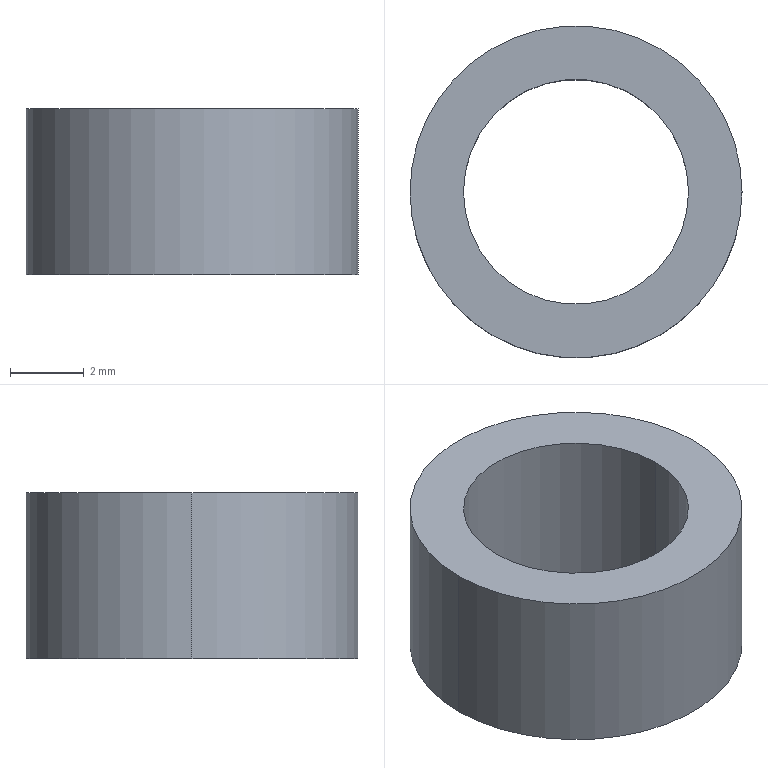Part | NX | features BREP 1 | 1 solid | 6 faces | box 9 x 9 x 4.5 mm | volume 154.767 mm3 | cylinder 4 | plane 2 | commonest cylinder face diameters 6.1 x2 9 x2
STEP:
#1=CARTESIAN_POINT('',(3.05,0.,4.5));
#2=VERTEX_POINT('',#1);
#3=CARTESIAN_POINT('',(3.05,0.,0.));
#4=VERTEX_POINT('',#3);
#5=CARTESIAN_POINT('',(3.05,0.,4.5));
#6=DIRECTION('',(0.,0.,-1.));
#7=VECTOR('',#6,1000.);
#8=LINE('',#5,#7);
#9=EDGE_CURVE('',#2,#4,#8,.T.);
#10=ORIENTED_EDGE('',*,*,#9,.F.);
#11=CARTESIAN_POINT('',(-3.05,0.,4.5));
#12=VERTEX_POINT('',#11);
#13=CARTESIAN_POINT('',(0.,0.,4.5));
#14=DIRECTION('',(0.,0.,1.));
#15=DIRECTION('',(1.,0.,0.));
#16=AXIS2_PLACEMENT_3D('',#13,#14,#15);
#17=CIRCLE('',#16,3.05);
#18=EDGE_CURVE('',#2,#12,#17,.T.);
#19=ORIENTED_EDGE('',*,*,#18,.T.);
#20=CARTESIAN_POINT('',(-3.05,0.,0.));
#21=VERTEX_POINT('',#20);
#22=CARTESIAN_POINT('',(-3.05,0.,4.5));
#23=DIRECTION('',(0.,0.,-1.));
#24=VECTOR('',#23,1000.);
#25=LINE('',#22,#24);
#26=EDGE_CURVE('',#12,#21,#25,.T.);
#27=ORIENTED_EDGE('',*,*,#26,.T.);
#28=CARTESIAN_POINT('',(0.,0.,0.));
#29=DIRECTION('',(0.,0.,1.));
#30=DIRECTION('',(1.,0.,0.));
#31=AXIS2_PLACEMENT_3D('',#28,#29,#30);
#32=CIRCLE('',#31,3.05);
#33=EDGE_CURVE('',#4,#21,#32,.T.);
#34=ORIENTED_EDGE('',*,*,#33,.F.);
#35=EDGE_LOOP('',(#10,#19,#27,#34));
#36=FACE_BOUND('',#35,.T.);
#37=CARTESIAN_POINT('',(0.,0.,4.5));
#38=DIRECTION('',(0.,0.,-1.));
#39=DIRECTION('',(-1.,0.,0.));
#40=AXIS2_PLACEMENT_3D('',#37,#38,#39);
#41=CYLINDRICAL_SURFACE('',#40,3.05);
#42=ADVANCED_FACE('',(#36),#41,.F.);
#43=CARTESIAN_POINT('',(4.5,0.,4.5));
#44=VERTEX_POINT('',#43);
#45=CARTESIAN_POINT('',(4.5,0.,0.));
#46=VERTEX_POINT('',#45);
#47=CARTESIAN_POINT('',(4.5,0.,4.5));
#48=DIRECTION('',(0.,0.,-1.));
#49=VECTOR('',#48,1000.);
#50=LINE('',#47,#49);
#51=EDGE_CURVE('',#44,#46,#50,.T.);
#52=ORIENTED_EDGE('',*,*,#51,.F.);
#53=CARTESIAN_POINT('',(-4.5,0.,4.5));
#54=VERTEX_POINT('',#53);
#55=CARTESIAN_POINT('',(0.,0.,4.5));
#56=DIRECTION('',(0.,0.,1.));
#57=DIRECTION('',(1.,0.,0.));
#58=AXIS2_PLACEMENT_3D('',#55,#56,#57);
#59=CIRCLE('',#58,4.5);
#60=EDGE_CURVE('',#54,#44,#59,.T.);
#61=ORIENTED_EDGE('',*,*,#60,.F.);
#62=CARTESIAN_POINT('',(-4.5,0.,0.));
#63=VERTEX_POINT('',#62);
#64=CARTESIAN_POINT('',(-4.5,0.,4.5));
#65=DIRECTION('',(0.,0.,-1.));
#66=VECTOR('',#65,1000.);
#67=LINE('',#64,#66);
#68=EDGE_CURVE('',#54,#63,#67,.T.);
#69=ORIENTED_EDGE('',*,*,#68,.T.);
#70=CARTESIAN_POINT('',(0.,0.,0.));
#71=DIRECTION('',(0.,0.,1.));
#72=DIRECTION('',(1.,0.,0.));
#73=AXIS2_PLACEMENT_3D('',#70,#71,#72);
#74=CIRCLE('',#73,4.5);
#75=EDGE_CURVE('',#63,#46,#74,.T.);
#76=ORIENTED_EDGE('',*,*,#75,.T.);
#77=EDGE_LOOP('',(#52,#61,#69,#76));
#78=FACE_BOUND('',#77,.T.);
#79=CARTESIAN_POINT('',(0.,0.,4.5));
#80=DIRECTION('',(0.,0.,-1.));
#81=DIRECTION('',(-1.,0.,0.));
#82=AXIS2_PLACEMENT_3D('',#79,#80,#81);
#83=CYLINDRICAL_SURFACE('',#82,4.5);
#84=ADVANCED_FACE('',(#78),#83,.T.);
#85=CARTESIAN_POINT('',(0.,0.,0.));
#86=DIRECTION('',(0.,0.,1.));
#87=DIRECTION('',(1.,0.,0.));
#88=AXIS2_PLACEMENT_3D('',#85,#86,#87);
#89=CIRCLE('',#88,3.05);
#90=EDGE_CURVE('',#21,#4,#89,.T.);
#91=ORIENTED_EDGE('',*,*,#90,.T.);
#92=ORIENTED_EDGE('',*,*,#33,.T.);
#93=EDGE_LOOP('',(#91,#92));
#94=FACE_BOUND('',#93,.T.);
#95=ORIENTED_EDGE('',*,*,#75,.F.);
#96=CARTESIAN_POINT('',(0.,0.,0.));
#97=DIRECTION('',(0.,0.,1.));
#98=DIRECTION('',(1.,0.,0.));
#99=AXIS2_PLACEMENT_3D('',#96,#97,#98);
#100=CIRCLE('',#99,4.5);
#101=EDGE_CURVE('',#46,#63,#100,.T.);
#102=ORIENTED_EDGE('',*,*,#101,.F.);
#103=EDGE_LOOP('',(#95,#102));
#104=FACE_BOUND('',#103,.T.);
#105=CARTESIAN_POINT('',(0.,0.,0.));
#106=DIRECTION('',(0.,0.,1.));
#107=DIRECTION('',(1.,0.,0.));
#108=AXIS2_PLACEMENT_3D('',#105,#106,#107);
#109=PLANE('',#108);
#110=ADVANCED_FACE('',(#94,#104),#109,.F.);
#111=CARTESIAN_POINT('',(0.,0.,4.5));
#112=DIRECTION('',(0.,0.,1.));
#113=DIRECTION('',(1.,0.,0.));
#114=AXIS2_PLACEMENT_3D('',#111,#112,#113);
#115=CIRCLE('',#114,3.05);
#116=EDGE_CURVE('',#12,#2,#115,.T.);
#117=ORIENTED_EDGE('',*,*,#116,.F.);
#118=ORIENTED_EDGE('',*,*,#18,.F.);
#119=EDGE_LOOP('',(#117,#118));
#120=FACE_BOUND('',#119,.T.);
#121=ORIENTED_EDGE('',*,*,#60,.T.);
#122=CARTESIAN_POINT('',(0.,0.,4.5));
#123=DIRECTION('',(0.,0.,1.));
#124=DIRECTION('',(1.,0.,0.));
#125=AXIS2_PLACEMENT_3D('',#122,#123,#124);
#126=CIRCLE('',#125,4.5);
#127=EDGE_CURVE('',#44,#54,#126,.T.);
#128=ORIENTED_EDGE('',*,*,#127,.T.);
#129=EDGE_LOOP('',(#121,#128));
#130=FACE_BOUND('',#129,.T.);
#131=CARTESIAN_POINT('',(0.,0.,4.5));
#132=DIRECTION('',(0.,0.,1.));
#133=DIRECTION('',(1.,0.,0.));
#134=AXIS2_PLACEMENT_3D('',#131,#132,#133);
#135=PLANE('',#134);
#136=ADVANCED_FACE('',(#120,#130),#135,.T.);
#137=ORIENTED_EDGE('',*,*,#127,.F.);
#138=ORIENTED_EDGE('',*,*,#51,.T.);
#139=ORIENTED_EDGE('',*,*,#101,.T.);
#140=ORIENTED_EDGE('',*,*,#68,.F.);
#141=EDGE_LOOP('',(#137,#138,#139,#140));
#142=FACE_BOUND('',#141,.T.);
#143=CARTESIAN_POINT('',(0.,0.,4.5));
#144=DIRECTION('',(0.,0.,-1.));
#145=DIRECTION('',(-1.,0.,0.));
#146=AXIS2_PLACEMENT_3D('',#143,#144,#145);
#147=CYLINDRICAL_SURFACE('',#146,4.5);
#148=ADVANCED_FACE('',(#142),#147,.T.);
#149=ORIENTED_EDGE('',*,*,#116,.T.);
#150=ORIENTED_EDGE('',*,*,#9,.T.);
#151=ORIENTED_EDGE('',*,*,#90,.F.);
#152=ORIENTED_EDGE('',*,*,#26,.F.);
#153=EDGE_LOOP('',(#149,#150,#151,#152));
#154=FACE_BOUND('',#153,.T.);
#155=CARTESIAN_POINT('',(0.,0.,4.5));
#156=DIRECTION('',(0.,0.,-1.));
#157=DIRECTION('',(-1.,0.,0.));
#158=AXIS2_PLACEMENT_3D('',#155,#156,#157);
#159=CYLINDRICAL_SURFACE('',#158,3.05);
#160=ADVANCED_FACE('',(#154),#159,.F.);
#161=CLOSED_SHELL('',(#42,#84,#110,#136,#148,#160));
#162=MANIFOLD_SOLID_BREP('',#161);
#163=(LENGTH_UNIT()NAMED_UNIT(*)SI_UNIT(.MILLI.,.METRE.));
#164=UNCERTAINTY_MEASURE_WITH_UNIT(LENGTH_MEASURE(0.00001),#163,'','');
#165=(NAMED_UNIT(*)PLANE_ANGLE_UNIT()SI_UNIT($,.RADIAN.));
#166=(NAMED_UNIT(*)SI_UNIT($,.STERADIAN.)SOLID_ANGLE_UNIT());
#167=(GEOMETRIC_REPRESENTATION_CONTEXT(3)GLOBAL_UNCERTAINTY_ASSIGNED_CONTEXT((#164))GLOBAL_UNIT_ASSIGNED_CONTEXT((#163,#165,#166))REPRESENTATION_CONTEXT('',''));
#168=ADVANCED_BREP_SHAPE_REPRESENTATION('',(#162),#167);